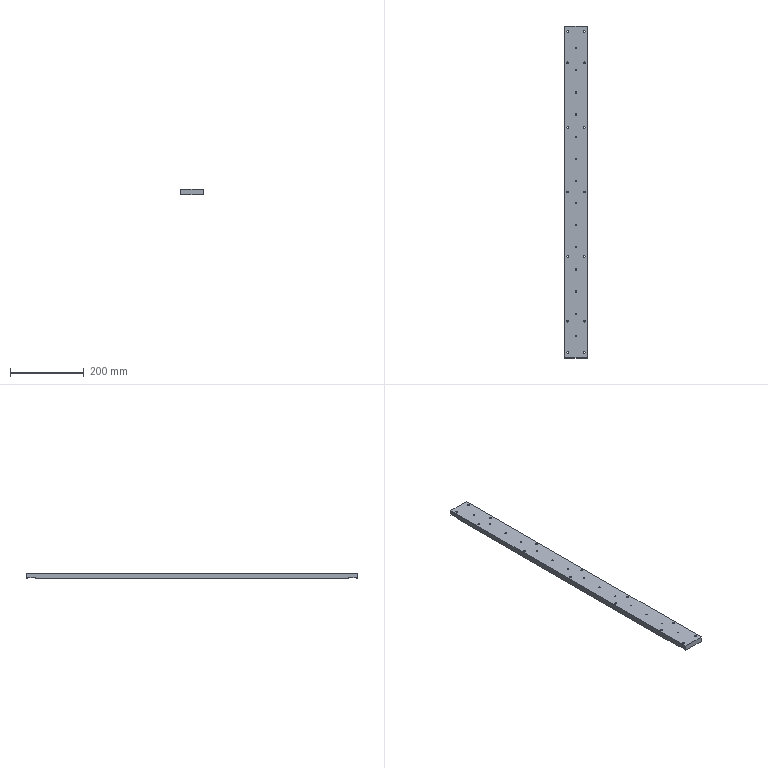Part | SolidWorks | features HoleWzd 4, ICE 2, LPattern 2, Extrusion 1 | 1 solid | 74 faces | box 60 x 900 x 15 mm | volume 771856 mm3 | cylinder 56 | plane 18 | commonest cylinder face diameters 3.3 x28 5 x28